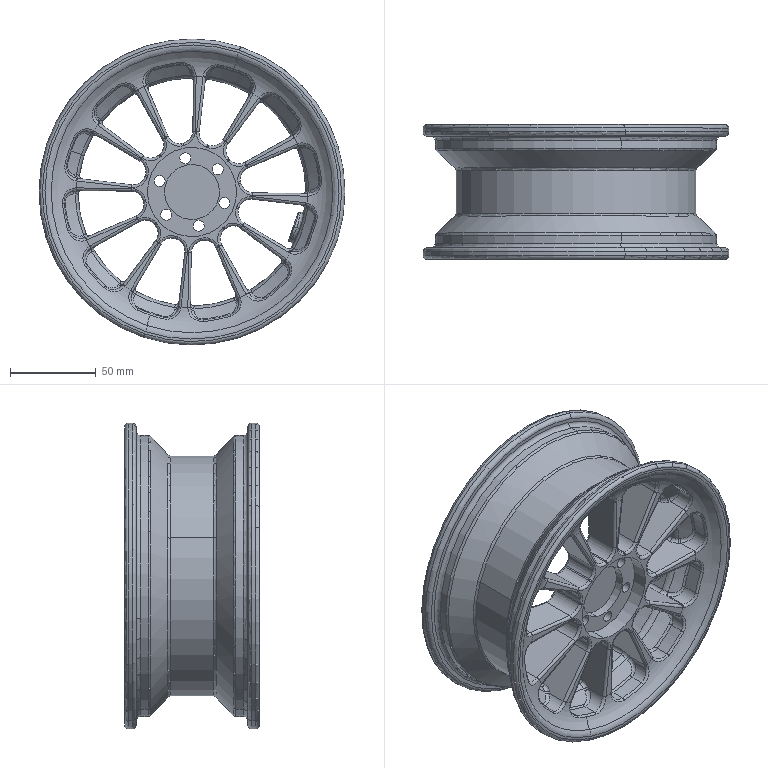Part | SolidWorks | features BaseBody 1 | 1 solid | 627 faces | box 178.5 x 78.5 x 178.5 mm | volume 311253 mm3 | cylinder 253 | torus 184 | spline 131 | plane 42 | cone 17 | commonest cylinder face diameters 14 x72 3 x70 4 x50 58 x13 6.4 x12 150 x12